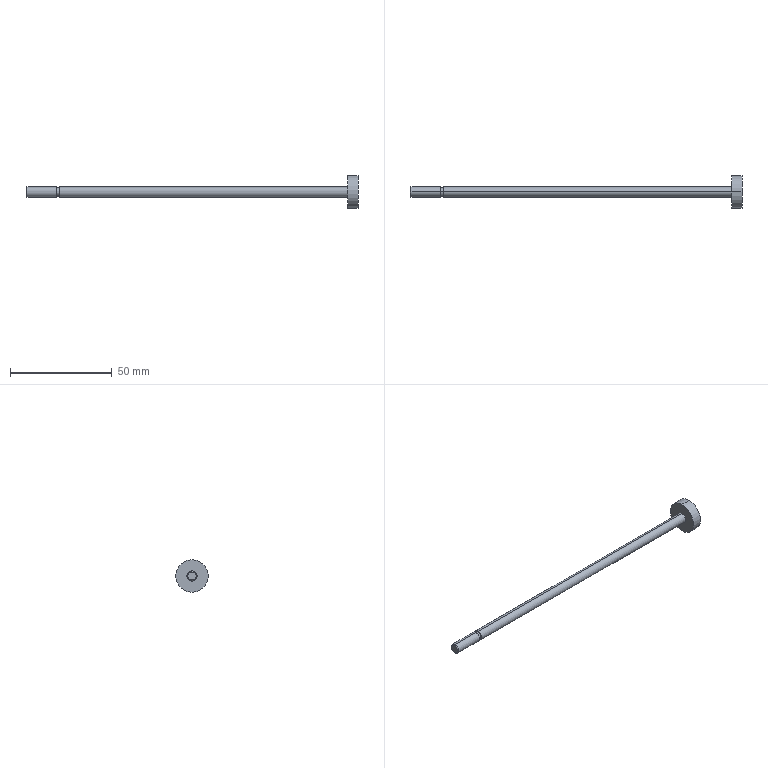Part | SolidWorks | features Revolution 1 | 1 solid | 15 faces | box 163.5 x 16 x 16 mm | volume 4106 mm3 | cylinder 8 | plane 5 | cone 2 | commonest cylinder face diameters 5 x4 4.13 x2 16 x2
STEP:
#1=CARTESIAN_POINT('',(130.5,0.,2.5));
#2=VERTEX_POINT('',#1);
#3=CARTESIAN_POINT('',(130.5,0.,-2.5));
#4=VERTEX_POINT('',#3);
#5=CARTESIAN_POINT('',(130.5,0.,0.));
#6=DIRECTION('',(-1.,0.,0.));
#7=DIRECTION('',(0.,0.,1.));
#8=AXIS2_PLACEMENT_3D('',#5,#6,#7);
#9=CIRCLE('',#8,2.5);
#10=EDGE_CURVE('',#2,#4,#9,.T.);
#11=ORIENTED_EDGE('',*,*,#10,.T.);
#12=CARTESIAN_POINT('',(-11.5,0.,-2.5));
#13=VERTEX_POINT('',#12);
#14=CARTESIAN_POINT('',(135.5,0.,-2.5));
#15=DIRECTION('',(-1.,0.,0.));
#16=VECTOR('',#15,1000.);
#17=LINE('',#14,#16);
#18=EDGE_CURVE('',#4,#13,#17,.T.);
#19=ORIENTED_EDGE('',*,*,#18,.T.);
#20=CARTESIAN_POINT('',(-11.5,0.,2.5));
#21=VERTEX_POINT('',#20);
#22=CARTESIAN_POINT('',(-11.5,0.,0.));
#23=DIRECTION('',(-1.,0.,0.));
#24=DIRECTION('',(0.,0.,1.));
#25=AXIS2_PLACEMENT_3D('',#22,#23,#24);
#26=CIRCLE('',#25,2.5);
#27=EDGE_CURVE('',#21,#13,#26,.T.);
#28=ORIENTED_EDGE('',*,*,#27,.F.);
#29=CARTESIAN_POINT('',(135.5,0.,2.5));
#30=DIRECTION('',(-1.,0.,0.));
#31=VECTOR('',#30,1000.);
#32=LINE('',#29,#31);
#33=EDGE_CURVE('',#2,#21,#32,.T.);
#34=ORIENTED_EDGE('',*,*,#33,.F.);
#35=EDGE_LOOP('',(#11,#19,#28,#34));
#36=FACE_OUTER_BOUND('',#35,.T.);
#37=CARTESIAN_POINT('',(135.5,0.,0.));
#38=DIRECTION('',(-1.,0.,0.));
#39=DIRECTION('',(0.,0.,1.));
#40=AXIS2_PLACEMENT_3D('',#37,#38,#39);
#41=CYLINDRICAL_SURFACE('',#40,2.5);
#42=ADVANCED_FACE('',(#36),#41,.T.);
#43=CARTESIAN_POINT('',(-11.5,0.,2.065));
#44=VERTEX_POINT('',#43);
#45=CARTESIAN_POINT('',(-11.5,0.,-2.065));
#46=VERTEX_POINT('',#45);
#47=CARTESIAN_POINT('',(-11.5,0.,0.));
#48=DIRECTION('',(-1.,0.,0.));
#49=DIRECTION('',(0.,0.,1.));
#50=AXIS2_PLACEMENT_3D('',#47,#48,#49);
#51=CIRCLE('',#50,2.065);
#52=EDGE_CURVE('',#44,#46,#51,.T.);
#53=ORIENTED_EDGE('',*,*,#52,.T.);
#54=CARTESIAN_POINT('',(-13.,0.,-2.065));
#55=VERTEX_POINT('',#54);
#56=CARTESIAN_POINT('',(135.5,0.,-2.065));
#57=DIRECTION('',(-1.,0.,0.));
#58=VECTOR('',#57,1000.);
#59=LINE('',#56,#58);
#60=EDGE_CURVE('',#46,#55,#59,.T.);
#61=ORIENTED_EDGE('',*,*,#60,.T.);
#62=CARTESIAN_POINT('',(-13.,0.,2.065));
#63=VERTEX_POINT('',#62);
#64=CARTESIAN_POINT('',(-13.,0.,0.));
#65=DIRECTION('',(-1.,0.,0.));
#66=DIRECTION('',(0.,0.,1.));
#67=AXIS2_PLACEMENT_3D('',#64,#65,#66);
#68=CIRCLE('',#67,2.065);
#69=EDGE_CURVE('',#63,#55,#68,.T.);
#70=ORIENTED_EDGE('',*,*,#69,.F.);
#71=CARTESIAN_POINT('',(135.5,0.,2.065));
#72=DIRECTION('',(-1.,0.,0.));
#73=VECTOR('',#72,1000.);
#74=LINE('',#71,#73);
#75=EDGE_CURVE('',#44,#63,#74,.T.);
#76=ORIENTED_EDGE('',*,*,#75,.F.);
#77=EDGE_LOOP('',(#53,#61,#70,#76));
#78=FACE_OUTER_BOUND('',#77,.T.);
#79=CARTESIAN_POINT('',(135.5,0.,0.));
#80=DIRECTION('',(-1.,0.,0.));
#81=DIRECTION('',(0.,0.,1.));
#82=AXIS2_PLACEMENT_3D('',#79,#80,#81);
#83=CYLINDRICAL_SURFACE('',#82,2.065);
#84=ADVANCED_FACE('',(#78),#83,.T.);
#85=CARTESIAN_POINT('',(-13.,0.,2.5));
#86=VERTEX_POINT('',#85);
#87=CARTESIAN_POINT('',(-13.,0.,-2.5));
#88=VERTEX_POINT('',#87);
#89=CARTESIAN_POINT('',(-13.,0.,0.));
#90=DIRECTION('',(-1.,0.,0.));
#91=DIRECTION('',(0.,0.,1.));
#92=AXIS2_PLACEMENT_3D('',#89,#90,#91);
#93=CIRCLE('',#92,2.5);
#94=EDGE_CURVE('',#86,#88,#93,.T.);
#95=ORIENTED_EDGE('',*,*,#94,.T.);
#96=CARTESIAN_POINT('',(-27.509,0.,-2.5));
#97=VERTEX_POINT('',#96);
#98=CARTESIAN_POINT('',(135.5,0.,-2.5));
#99=DIRECTION('',(-1.,0.,0.));
#100=VECTOR('',#99,1000.);
#101=LINE('',#98,#100);
#102=EDGE_CURVE('',#88,#97,#101,.T.);
#103=ORIENTED_EDGE('',*,*,#102,.T.);
#104=CARTESIAN_POINT('',(-27.509,0.,2.5));
#105=VERTEX_POINT('',#104);
#106=CARTESIAN_POINT('',(-27.509,0.,0.));
#107=DIRECTION('',(-1.,0.,0.));
#108=DIRECTION('',(0.,0.,1.));
#109=AXIS2_PLACEMENT_3D('',#106,#107,#108);
#110=CIRCLE('',#109,2.5);
#111=EDGE_CURVE('',#105,#97,#110,.T.);
#112=ORIENTED_EDGE('',*,*,#111,.F.);
#113=CARTESIAN_POINT('',(135.5,0.,2.5));
#114=DIRECTION('',(-1.,0.,0.));
#115=VECTOR('',#114,1000.);
#116=LINE('',#113,#115);
#117=EDGE_CURVE('',#86,#105,#116,.T.);
#118=ORIENTED_EDGE('',*,*,#117,.F.);
#119=EDGE_LOOP('',(#95,#103,#112,#118));
#120=FACE_OUTER_BOUND('',#119,.T.);
#121=CARTESIAN_POINT('',(135.5,0.,0.));
#122=DIRECTION('',(-1.,0.,0.));
#123=DIRECTION('',(0.,0.,1.));
#124=AXIS2_PLACEMENT_3D('',#121,#122,#123);
#125=CYLINDRICAL_SURFACE('',#124,2.5);
#126=ADVANCED_FACE('',(#120),#125,.T.);
#127=CARTESIAN_POINT('',(-28.,0.,2.009));
#128=VERTEX_POINT('',#127);
#129=CARTESIAN_POINT('',(-28.,0.,-2.009));
#130=VERTEX_POINT('',#129);
#131=CARTESIAN_POINT('',(-28.,0.,0.));
#132=DIRECTION('',(-1.,0.,0.));
#133=DIRECTION('',(0.,0.,1.));
#134=AXIS2_PLACEMENT_3D('',#131,#132,#133);
#135=CIRCLE('',#134,2.009);
#136=EDGE_CURVE('',#128,#130,#135,.T.);
#137=ORIENTED_EDGE('',*,*,#136,.F.);
#138=CARTESIAN_POINT('',(-28.,0.,2.009));
#139=DIRECTION('',(0.7071,0.,0.7071));
#140=VECTOR('',#139,1000.);
#141=LINE('',#138,#140);
#142=EDGE_CURVE('',#128,#105,#141,.T.);
#143=ORIENTED_EDGE('',*,*,#142,.T.);
#144=ORIENTED_EDGE('',*,*,#111,.T.);
#145=CARTESIAN_POINT('',(-28.,0.,-2.009));
#146=DIRECTION('',(0.7071,0.,-0.7071));
#147=VECTOR('',#146,1000.);
#148=LINE('',#145,#147);
#149=EDGE_CURVE('',#130,#97,#148,.T.);
#150=ORIENTED_EDGE('',*,*,#149,.F.);
#151=EDGE_LOOP('',(#137,#143,#144,#150));
#152=FACE_OUTER_BOUND('',#151,.T.);
#153=CARTESIAN_POINT('',(-28.,0.,0.));
#154=DIRECTION('',(1.,0.,0.));
#155=DIRECTION('',(0.,0.,-1.));
#156=AXIS2_PLACEMENT_3D('',#153,#154,#155);
#157=CONICAL_SURFACE('',#156,2.009,0.7854);
#158=ADVANCED_FACE('',(#152),#157,.T.);
#159=CARTESIAN_POINT('',(135.5,0.,8.));
#160=VERTEX_POINT('',#159);
#161=CARTESIAN_POINT('',(135.5,0.,-8.));
#162=VERTEX_POINT('',#161);
#163=CARTESIAN_POINT('',(135.5,0.,0.));
#164=DIRECTION('',(-1.,0.,0.));
#165=DIRECTION('',(0.,0.,1.));
#166=AXIS2_PLACEMENT_3D('',#163,#164,#165);
#167=CIRCLE('',#166,8.);
#168=EDGE_CURVE('',#160,#162,#167,.T.);
#169=ORIENTED_EDGE('',*,*,#168,.T.);
#170=CARTESIAN_POINT('',(130.5,0.,-8.));
#171=VERTEX_POINT('',#170);
#172=CARTESIAN_POINT('',(135.5,0.,-8.));
#173=DIRECTION('',(-1.,0.,0.));
#174=VECTOR('',#173,1000.);
#175=LINE('',#172,#174);
#176=EDGE_CURVE('',#162,#171,#175,.T.);
#177=ORIENTED_EDGE('',*,*,#176,.T.);
#178=CARTESIAN_POINT('',(130.5,0.,8.));
#179=VERTEX_POINT('',#178);
#180=CARTESIAN_POINT('',(130.5,0.,0.));
#181=DIRECTION('',(-1.,0.,0.));
#182=DIRECTION('',(0.,0.,1.));
#183=AXIS2_PLACEMENT_3D('',#180,#181,#182);
#184=CIRCLE('',#183,8.);
#185=EDGE_CURVE('',#179,#171,#184,.T.);
#186=ORIENTED_EDGE('',*,*,#185,.F.);
#187=CARTESIAN_POINT('',(135.5,0.,8.));
#188=DIRECTION('',(-1.,0.,0.));
#189=VECTOR('',#188,1000.);
#190=LINE('',#187,#189);
#191=EDGE_CURVE('',#160,#179,#190,.T.);
#192=ORIENTED_EDGE('',*,*,#191,.F.);
#193=EDGE_LOOP('',(#169,#177,#186,#192));
#194=FACE_OUTER_BOUND('',#193,.T.);
#195=CARTESIAN_POINT('',(135.5,0.,0.));
#196=DIRECTION('',(-1.,0.,0.));
#197=DIRECTION('',(0.,0.,1.));
#198=AXIS2_PLACEMENT_3D('',#195,#196,#197);
#199=CYLINDRICAL_SURFACE('',#198,8.);
#200=ADVANCED_FACE('',(#194),#199,.T.);
#201=ORIENTED_EDGE('',*,*,#176,.F.);
#202=CARTESIAN_POINT('',(135.5,0.,0.));
#203=DIRECTION('',(-1.,0.,0.));
#204=DIRECTION('',(0.,0.,1.));
#205=AXIS2_PLACEMENT_3D('',#202,#203,#204);
#206=CIRCLE('',#205,8.);
#207=EDGE_CURVE('',#162,#160,#206,.T.);
#208=ORIENTED_EDGE('',*,*,#207,.T.);
#209=ORIENTED_EDGE('',*,*,#191,.T.);
#210=CARTESIAN_POINT('',(130.5,0.,0.));
#211=DIRECTION('',(-1.,0.,0.));
#212=DIRECTION('',(0.,0.,1.));
#213=AXIS2_PLACEMENT_3D('',#210,#211,#212);
#214=CIRCLE('',#213,8.);
#215=EDGE_CURVE('',#171,#179,#214,.T.);
#216=ORIENTED_EDGE('',*,*,#215,.F.);
#217=EDGE_LOOP('',(#201,#208,#209,#216));
#218=FACE_OUTER_BOUND('',#217,.T.);
#219=CARTESIAN_POINT('',(135.5,0.,0.));
#220=DIRECTION('',(-1.,0.,0.));
#221=DIRECTION('',(0.,0.,1.));
#222=AXIS2_PLACEMENT_3D('',#219,#220,#221);
#223=CYLINDRICAL_SURFACE('',#222,8.);
#224=ADVANCED_FACE('',(#218),#223,.T.);
#225=ORIENTED_EDGE('',*,*,#168,.F.);
#226=ORIENTED_EDGE('',*,*,#207,.F.);
#227=EDGE_LOOP('',(#225,#226));
#228=FACE_OUTER_BOUND('',#227,.T.);
#229=CARTESIAN_POINT('',(135.5,8.,0.));
#230=DIRECTION('',(1.,0.,0.));
#231=DIRECTION('',(0.,0.,-1.));
#232=AXIS2_PLACEMENT_3D('',#229,#230,#231);
#233=PLANE('',#232);
#234=ADVANCED_FACE('',(#228),#233,.T.);
#235=CARTESIAN_POINT('',(-28.,0.,0.));
#236=DIRECTION('',(-1.,0.,0.));
#237=DIRECTION('',(0.,0.,1.));
#238=AXIS2_PLACEMENT_3D('',#235,#236,#237);
#239=CIRCLE('',#238,2.009);
#240=EDGE_CURVE('',#130,#128,#239,.T.);
#241=ORIENTED_EDGE('',*,*,#240,.T.);
#242=ORIENTED_EDGE('',*,*,#136,.T.);
#243=EDGE_LOOP('',(#241,#242));
#244=FACE_OUTER_BOUND('',#243,.T.);
#245=CARTESIAN_POINT('',(-28.,0.,0.));
#246=DIRECTION('',(-1.,0.,0.));
#247=DIRECTION('',(0.,0.,1.));
#248=AXIS2_PLACEMENT_3D('',#245,#246,#247);
#249=PLANE('',#248);
#250=ADVANCED_FACE('',(#244),#249,.T.);
#251=ORIENTED_EDGE('',*,*,#142,.F.);
#252=ORIENTED_EDGE('',*,*,#240,.F.);
#253=ORIENTED_EDGE('',*,*,#149,.T.);
#254=CARTESIAN_POINT('',(-27.509,0.,0.));
#255=DIRECTION('',(-1.,0.,0.));
#256=DIRECTION('',(0.,0.,1.));
#257=AXIS2_PLACEMENT_3D('',#254,#255,#256);
#258=CIRCLE('',#257,2.5);
#259=EDGE_CURVE('',#97,#105,#258,.T.);
#260=ORIENTED_EDGE('',*,*,#259,.T.);
#261=EDGE_LOOP('',(#251,#252,#253,#260));
#262=FACE_OUTER_BOUND('',#261,.T.);
#263=CARTESIAN_POINT('',(-28.,0.,0.));
#264=DIRECTION('',(1.,0.,0.));
#265=DIRECTION('',(0.,0.,-1.));
#266=AXIS2_PLACEMENT_3D('',#263,#264,#265);
#267=CONICAL_SURFACE('',#266,2.009,0.7854);
#268=ADVANCED_FACE('',(#262),#267,.T.);
#269=ORIENTED_EDGE('',*,*,#102,.F.);
#270=CARTESIAN_POINT('',(-13.,0.,0.));
#271=DIRECTION('',(-1.,0.,0.));
#272=DIRECTION('',(0.,0.,1.));
#273=AXIS2_PLACEMENT_3D('',#270,#271,#272);
#274=CIRCLE('',#273,2.5);
#275=EDGE_CURVE('',#88,#86,#274,.T.);
#276=ORIENTED_EDGE('',*,*,#275,.T.);
#277=ORIENTED_EDGE('',*,*,#117,.T.);
#278=ORIENTED_EDGE('',*,*,#259,.F.);
#279=EDGE_LOOP('',(#269,#276,#277,#278));
#280=FACE_OUTER_BOUND('',#279,.T.);
#281=CARTESIAN_POINT('',(135.5,0.,0.));
#282=DIRECTION('',(-1.,0.,0.));
#283=DIRECTION('',(0.,0.,1.));
#284=AXIS2_PLACEMENT_3D('',#281,#282,#283);
#285=CYLINDRICAL_SURFACE('',#284,2.5);
#286=ADVANCED_FACE('',(#280),#285,.T.);
#287=ORIENTED_EDGE('',*,*,#69,.T.);
#288=CARTESIAN_POINT('',(-13.,0.,0.));
#289=DIRECTION('',(-1.,0.,0.));
#290=DIRECTION('',(0.,0.,1.));
#291=AXIS2_PLACEMENT_3D('',#288,#289,#290);
#292=CIRCLE('',#291,2.065);
#293=EDGE_CURVE('',#55,#63,#292,.T.);
#294=ORIENTED_EDGE('',*,*,#293,.T.);
#295=EDGE_LOOP('',(#287,#294));
#296=FACE_BOUND('',#295,.T.);
#297=ORIENTED_EDGE('',*,*,#94,.F.);
#298=ORIENTED_EDGE('',*,*,#275,.F.);
#299=EDGE_LOOP('',(#297,#298));
#300=FACE_OUTER_BOUND('',#299,.T.);
#301=CARTESIAN_POINT('',(-13.,2.5,0.));
#302=DIRECTION('',(1.,0.,0.));
#303=DIRECTION('',(0.,0.,-1.));
#304=AXIS2_PLACEMENT_3D('',#301,#302,#303);
#305=PLANE('',#304);
#306=ADVANCED_FACE('',(#296,#300),#305,.T.);
#307=ORIENTED_EDGE('',*,*,#60,.F.);
#308=CARTESIAN_POINT('',(-11.5,0.,0.));
#309=DIRECTION('',(-1.,0.,0.));
#310=DIRECTION('',(0.,0.,1.));
#311=AXIS2_PLACEMENT_3D('',#308,#309,#310);
#312=CIRCLE('',#311,2.065);
#313=EDGE_CURVE('',#46,#44,#312,.T.);
#314=ORIENTED_EDGE('',*,*,#313,.T.);
#315=ORIENTED_EDGE('',*,*,#75,.T.);
#316=ORIENTED_EDGE('',*,*,#293,.F.);
#317=EDGE_LOOP('',(#307,#314,#315,#316));
#318=FACE_OUTER_BOUND('',#317,.T.);
#319=CARTESIAN_POINT('',(135.5,0.,0.));
#320=DIRECTION('',(-1.,0.,0.));
#321=DIRECTION('',(0.,0.,1.));
#322=AXIS2_PLACEMENT_3D('',#319,#320,#321);
#323=CYLINDRICAL_SURFACE('',#322,2.065);
#324=ADVANCED_FACE('',(#318),#323,.T.);
#325=ORIENTED_EDGE('',*,*,#27,.T.);
#326=CARTESIAN_POINT('',(-11.5,0.,0.));
#327=DIRECTION('',(-1.,0.,0.));
#328=DIRECTION('',(0.,0.,1.));
#329=AXIS2_PLACEMENT_3D('',#326,#327,#328);
#330=CIRCLE('',#329,2.5);
#331=EDGE_CURVE('',#13,#21,#330,.T.);
#332=ORIENTED_EDGE('',*,*,#331,.T.);
#333=EDGE_LOOP('',(#325,#332));
#334=FACE_OUTER_BOUND('',#333,.T.);
#335=ORIENTED_EDGE('',*,*,#52,.F.);
#336=ORIENTED_EDGE('',*,*,#313,.F.);
#337=EDGE_LOOP('',(#335,#336));
#338=FACE_BOUND('',#337,.T.);
#339=CARTESIAN_POINT('',(-11.5,2.065,0.));
#340=DIRECTION('',(-1.,0.,0.));
#341=DIRECTION('',(0.,0.,1.));
#342=AXIS2_PLACEMENT_3D('',#339,#340,#341);
#343=PLANE('',#342);
#344=ADVANCED_FACE('',(#334,#338),#343,.T.);
#345=ORIENTED_EDGE('',*,*,#18,.F.);
#346=CARTESIAN_POINT('',(130.5,0.,0.));
#347=DIRECTION('',(-1.,0.,0.));
#348=DIRECTION('',(0.,0.,1.));
#349=AXIS2_PLACEMENT_3D('',#346,#347,#348);
#350=CIRCLE('',#349,2.5);
#351=EDGE_CURVE('',#4,#2,#350,.T.);
#352=ORIENTED_EDGE('',*,*,#351,.T.);
#353=ORIENTED_EDGE('',*,*,#33,.T.);
#354=ORIENTED_EDGE('',*,*,#331,.F.);
#355=EDGE_LOOP('',(#345,#352,#353,#354));
#356=FACE_OUTER_BOUND('',#355,.T.);
#357=CARTESIAN_POINT('',(135.5,0.,0.));
#358=DIRECTION('',(-1.,0.,0.));
#359=DIRECTION('',(0.,0.,1.));
#360=AXIS2_PLACEMENT_3D('',#357,#358,#359);
#361=CYLINDRICAL_SURFACE('',#360,2.5);
#362=ADVANCED_FACE('',(#356),#361,.T.);
#363=ORIENTED_EDGE('',*,*,#185,.T.);
#364=ORIENTED_EDGE('',*,*,#215,.T.);
#365=EDGE_LOOP('',(#363,#364));
#366=FACE_OUTER_BOUND('',#365,.T.);
#367=ORIENTED_EDGE('',*,*,#10,.F.);
#368=ORIENTED_EDGE('',*,*,#351,.F.);
#369=EDGE_LOOP('',(#367,#368));
#370=FACE_BOUND('',#369,.T.);
#371=CARTESIAN_POINT('',(130.5,2.5,0.));
#372=DIRECTION('',(-1.,0.,0.));
#373=DIRECTION('',(0.,0.,1.));
#374=AXIS2_PLACEMENT_3D('',#371,#372,#373);
#375=PLANE('',#374);
#376=ADVANCED_FACE('',(#366,#370),#375,.T.);
#377=CLOSED_SHELL('',(#42,#84,#126,#158,#200,#224,#234,#250,#268,#286,#306,#324,#344,#362,#376));
#378=MANIFOLD_SOLID_BREP('',#377);
#379=CARTESIAN_POINT('',(0.,0.,0.));
#380=DIRECTION('',(0.,0.,1.));
#381=DIRECTION('',(1.,0.,0.));
#382=AXIS2_PLACEMENT_3D('',#379,#380,#381);
#383=(LENGTH_UNIT()NAMED_UNIT(*)SI_UNIT(.MILLI.,.METRE.));
#384=UNCERTAINTY_MEASURE_WITH_UNIT(LENGTH_MEASURE(0.00001),#383,'','');
#385=(NAMED_UNIT(*)PLANE_ANGLE_UNIT()SI_UNIT($,.RADIAN.));
#386=(NAMED_UNIT(*)SI_UNIT($,.STERADIAN.)SOLID_ANGLE_UNIT());
#387=(GEOMETRIC_REPRESENTATION_CONTEXT(3)GLOBAL_UNCERTAINTY_ASSIGNED_CONTEXT((#384))GLOBAL_UNIT_ASSIGNED_CONTEXT((#383,#385,#386))REPRESENTATION_CONTEXT('',''));
#388=ADVANCED_BREP_SHAPE_REPRESENTATION('',(#378,#382),#387);